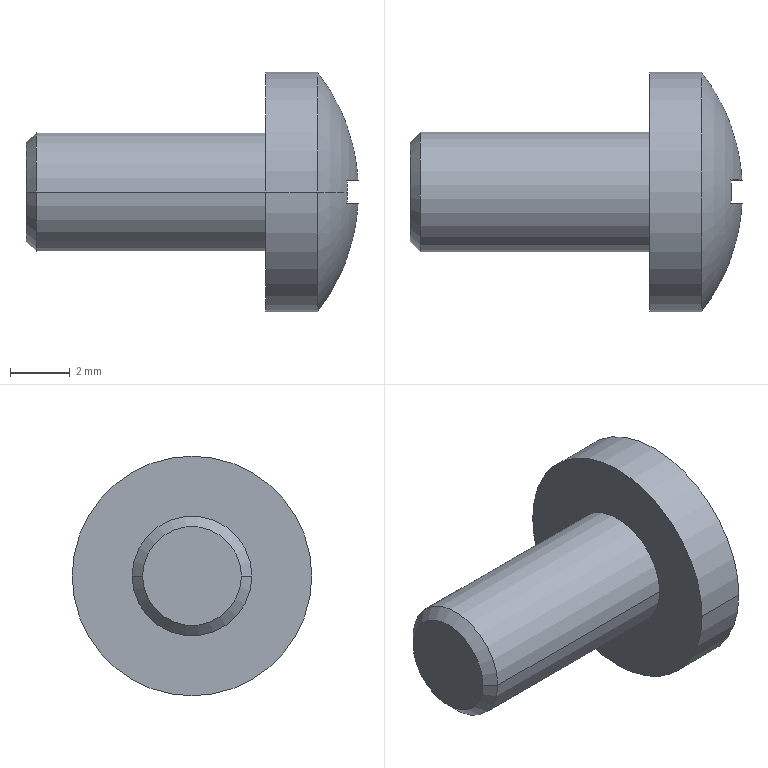Part | STEP file | SOLID | 1 solid | 23 faces | box 11.088 x 8 x 8 mm | volume 218.221 mm3 | plane 15 | cylinder 4 | sphere 2 | cone 2 | commonest cylinder face diameters 4 x2 8 x2